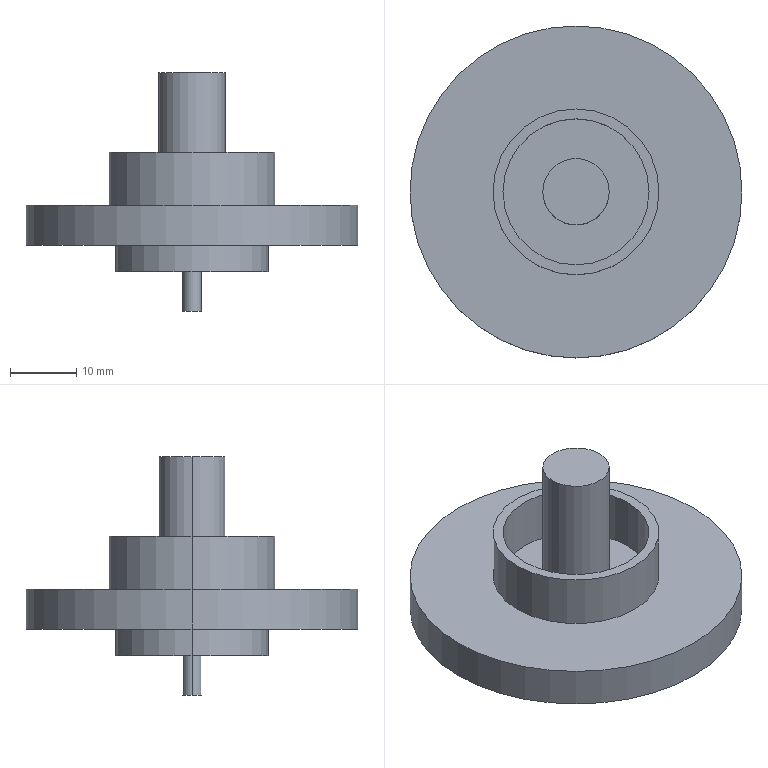Part | SolidWorks | features ICE 4, Extrusion 1 | 1 solid | 22 faces | box 50 x 50 x 36 mm | volume 14585 mm3 | cylinder 14 | plane 8 | commonest cylinder face diameters 2.85 x2 10 x2 20.95 x2 22 x2 23 x2 25 x2
STEP:
#1=CARTESIAN_POINT('',(-1.425,0.,-10.));
#2=VERTEX_POINT('',#1);
#3=CARTESIAN_POINT('',(1.425,0.,-10.));
#4=VERTEX_POINT('',#3);
#5=CARTESIAN_POINT('',(0.,0.,-10.));
#6=DIRECTION('',(0.,0.,-1.));
#7=DIRECTION('',(-1.,0.,0.));
#8=AXIS2_PLACEMENT_3D('',#5,#6,#7);
#9=CIRCLE('',#8,1.425);
#10=EDGE_CURVE('',#2,#4,#9,.T.);
#11=ORIENTED_EDGE('',*,*,#10,.F.);
#12=CARTESIAN_POINT('',(-1.425,0.,0.));
#13=VERTEX_POINT('',#12);
#14=CARTESIAN_POINT('',(-1.425,0.,-10.));
#15=DIRECTION('',(0.,0.,1.));
#16=VECTOR('',#15,1000.);
#17=LINE('',#14,#16);
#18=EDGE_CURVE('',#2,#13,#17,.T.);
#19=ORIENTED_EDGE('',*,*,#18,.T.);
#20=CARTESIAN_POINT('',(1.425,0.,0.));
#21=VERTEX_POINT('',#20);
#22=CARTESIAN_POINT('',(0.,0.,0.));
#23=DIRECTION('',(0.,0.,-1.));
#24=DIRECTION('',(1.,0.,0.));
#25=AXIS2_PLACEMENT_3D('',#22,#23,#24);
#26=CIRCLE('',#25,1.425);
#27=EDGE_CURVE('',#13,#21,#26,.T.);
#28=ORIENTED_EDGE('',*,*,#27,.T.);
#29=CARTESIAN_POINT('',(1.425,0.,-10.));
#30=DIRECTION('',(0.,0.,1.));
#31=VECTOR('',#30,1000.);
#32=LINE('',#29,#31);
#33=EDGE_CURVE('',#4,#21,#32,.T.);
#34=ORIENTED_EDGE('',*,*,#33,.F.);
#35=EDGE_LOOP('',(#11,#19,#28,#34));
#36=FACE_OUTER_BOUND('',#35,.T.);
#37=CARTESIAN_POINT('',(0.,0.,-10.));
#38=DIRECTION('',(0.,0.,1.));
#39=DIRECTION('',(1.,0.,0.));
#40=AXIS2_PLACEMENT_3D('',#37,#38,#39);
#41=CYLINDRICAL_SURFACE('',#40,1.425);
#42=ADVANCED_FACE('',(#36),#41,.T.);
#43=CARTESIAN_POINT('',(10.475,0.,-4.));
#44=VERTEX_POINT('',#43);
#45=CARTESIAN_POINT('',(-10.475,0.,-4.));
#46=VERTEX_POINT('',#45);
#47=CARTESIAN_POINT('',(0.,0.,-4.));
#48=DIRECTION('',(0.,0.,-1.));
#49=DIRECTION('',(-1.,0.,0.));
#50=AXIS2_PLACEMENT_3D('',#47,#48,#49);
#51=CIRCLE('',#50,10.475);
#52=EDGE_CURVE('',#44,#46,#51,.T.);
#53=ORIENTED_EDGE('',*,*,#52,.T.);
#54=CARTESIAN_POINT('',(-10.475,0.,0.));
#55=VERTEX_POINT('',#54);
#56=CARTESIAN_POINT('',(-10.475,0.,-4.));
#57=DIRECTION('',(0.,0.,1.));
#58=VECTOR('',#57,1000.);
#59=LINE('',#56,#58);
#60=EDGE_CURVE('',#46,#55,#59,.T.);
#61=ORIENTED_EDGE('',*,*,#60,.T.);
#62=CARTESIAN_POINT('',(10.475,0.,0.));
#63=VERTEX_POINT('',#62);
#64=CARTESIAN_POINT('',(0.,0.,0.));
#65=DIRECTION('',(0.,0.,-1.));
#66=DIRECTION('',(-1.,0.,0.));
#67=AXIS2_PLACEMENT_3D('',#64,#65,#66);
#68=CIRCLE('',#67,10.475);
#69=EDGE_CURVE('',#63,#55,#68,.T.);
#70=ORIENTED_EDGE('',*,*,#69,.F.);
#71=CARTESIAN_POINT('',(10.475,0.,-4.));
#72=DIRECTION('',(0.,0.,1.));
#73=VECTOR('',#72,1000.);
#74=LINE('',#71,#73);
#75=EDGE_CURVE('',#44,#63,#74,.T.);
#76=ORIENTED_EDGE('',*,*,#75,.F.);
#77=EDGE_LOOP('',(#53,#61,#70,#76));
#78=FACE_OUTER_BOUND('',#77,.T.);
#79=CARTESIAN_POINT('',(0.,0.,-4.));
#80=DIRECTION('',(0.,0.,1.));
#81=DIRECTION('',(1.,0.,0.));
#82=AXIS2_PLACEMENT_3D('',#79,#80,#81);
#83=CYLINDRICAL_SURFACE('',#82,10.475);
#84=ADVANCED_FACE('',(#78),#83,.F.);
#85=CARTESIAN_POINT('',(-11.5,0.,-4.));
#86=VERTEX_POINT('',#85);
#87=CARTESIAN_POINT('',(11.5,0.,-4.));
#88=VERTEX_POINT('',#87);
#89=CARTESIAN_POINT('',(0.,0.,-4.));
#90=DIRECTION('',(0.,0.,-1.));
#91=DIRECTION('',(-1.,0.,0.));
#92=AXIS2_PLACEMENT_3D('',#89,#90,#91);
#93=CIRCLE('',#92,11.5);
#94=EDGE_CURVE('',#86,#88,#93,.T.);
#95=ORIENTED_EDGE('',*,*,#94,.F.);
#96=CARTESIAN_POINT('',(-11.5,0.,0.));
#97=VERTEX_POINT('',#96);
#98=CARTESIAN_POINT('',(-11.5,0.,-4.));
#99=DIRECTION('',(0.,0.,1.));
#100=VECTOR('',#99,1000.);
#101=LINE('',#98,#100);
#102=EDGE_CURVE('',#86,#97,#101,.T.);
#103=ORIENTED_EDGE('',*,*,#102,.T.);
#104=CARTESIAN_POINT('',(11.5,0.,0.));
#105=VERTEX_POINT('',#104);
#106=CARTESIAN_POINT('',(0.,0.,0.));
#107=DIRECTION('',(0.,0.,-1.));
#108=DIRECTION('',(1.,0.,0.));
#109=AXIS2_PLACEMENT_3D('',#106,#107,#108);
#110=CIRCLE('',#109,11.5);
#111=EDGE_CURVE('',#97,#105,#110,.T.);
#112=ORIENTED_EDGE('',*,*,#111,.T.);
#113=CARTESIAN_POINT('',(11.5,0.,-4.));
#114=DIRECTION('',(0.,0.,1.));
#115=VECTOR('',#114,1000.);
#116=LINE('',#113,#115);
#117=EDGE_CURVE('',#88,#105,#116,.T.);
#118=ORIENTED_EDGE('',*,*,#117,.F.);
#119=EDGE_LOOP('',(#95,#103,#112,#118));
#120=FACE_OUTER_BOUND('',#119,.T.);
#121=CARTESIAN_POINT('',(0.,0.,-4.));
#122=DIRECTION('',(0.,0.,1.));
#123=DIRECTION('',(1.,0.,0.));
#124=AXIS2_PLACEMENT_3D('',#121,#122,#123);
#125=CYLINDRICAL_SURFACE('',#124,11.5);
#126=ADVANCED_FACE('',(#120),#125,.T.);
#127=CARTESIAN_POINT('',(5.,0.,26.));
#128=VERTEX_POINT('',#127);
#129=CARTESIAN_POINT('',(-5.,0.,26.));
#130=VERTEX_POINT('',#129);
#131=CARTESIAN_POINT('',(0.,0.,26.));
#132=DIRECTION('',(0.,0.,1.));
#133=DIRECTION('',(1.,0.,0.));
#134=AXIS2_PLACEMENT_3D('',#131,#132,#133);
#135=CIRCLE('',#134,5.);
#136=EDGE_CURVE('',#128,#130,#135,.T.);
#137=ORIENTED_EDGE('',*,*,#136,.F.);
#138=CARTESIAN_POINT('',(5.,0.,6.));
#139=VERTEX_POINT('',#138);
#140=CARTESIAN_POINT('',(5.,0.,26.));
#141=DIRECTION('',(0.,0.,-1.));
#142=VECTOR('',#141,1000.);
#143=LINE('',#140,#142);
#144=EDGE_CURVE('',#128,#139,#143,.T.);
#145=ORIENTED_EDGE('',*,*,#144,.T.);
#146=CARTESIAN_POINT('',(-5.,0.,6.));
#147=VERTEX_POINT('',#146);
#148=CARTESIAN_POINT('',(0.,0.,6.));
#149=DIRECTION('',(0.,0.,1.));
#150=DIRECTION('',(1.,0.,0.));
#151=AXIS2_PLACEMENT_3D('',#148,#149,#150);
#152=CIRCLE('',#151,5.);
#153=EDGE_CURVE('',#139,#147,#152,.T.);
#154=ORIENTED_EDGE('',*,*,#153,.T.);
#155=CARTESIAN_POINT('',(-5.,0.,26.));
#156=DIRECTION('',(0.,0.,-1.));
#157=VECTOR('',#156,1000.);
#158=LINE('',#155,#157);
#159=EDGE_CURVE('',#130,#147,#158,.T.);
#160=ORIENTED_EDGE('',*,*,#159,.F.);
#161=EDGE_LOOP('',(#137,#145,#154,#160));
#162=FACE_OUTER_BOUND('',#161,.T.);
#163=CARTESIAN_POINT('',(0.,0.,26.));
#164=DIRECTION('',(0.,0.,-1.));
#165=DIRECTION('',(-1.,0.,0.));
#166=AXIS2_PLACEMENT_3D('',#163,#164,#165);
#167=CYLINDRICAL_SURFACE('',#166,5.);
#168=ADVANCED_FACE('',(#162),#167,.T.);
#169=CARTESIAN_POINT('',(-11.,0.,14.));
#170=VERTEX_POINT('',#169);
#171=CARTESIAN_POINT('',(11.,0.,14.));
#172=VERTEX_POINT('',#171);
#173=CARTESIAN_POINT('',(0.,0.,14.));
#174=DIRECTION('',(0.,0.,1.));
#175=DIRECTION('',(1.,0.,0.));
#176=AXIS2_PLACEMENT_3D('',#173,#174,#175);
#177=CIRCLE('',#176,11.);
#178=EDGE_CURVE('',#170,#172,#177,.T.);
#179=ORIENTED_EDGE('',*,*,#178,.T.);
#180=CARTESIAN_POINT('',(11.,0.,6.));
#181=VERTEX_POINT('',#180);
#182=CARTESIAN_POINT('',(11.,0.,14.));
#183=DIRECTION('',(0.,0.,-1.));
#184=VECTOR('',#183,1000.);
#185=LINE('',#182,#184);
#186=EDGE_CURVE('',#172,#181,#185,.T.);
#187=ORIENTED_EDGE('',*,*,#186,.T.);
#188=CARTESIAN_POINT('',(-11.,0.,6.));
#189=VERTEX_POINT('',#188);
#190=CARTESIAN_POINT('',(0.,0.,6.));
#191=DIRECTION('',(0.,0.,-1.));
#192=DIRECTION('',(1.,0.,0.));
#193=AXIS2_PLACEMENT_3D('',#190,#191,#192);
#194=CIRCLE('',#193,11.);
#195=EDGE_CURVE('',#181,#189,#194,.T.);
#196=ORIENTED_EDGE('',*,*,#195,.T.);
#197=CARTESIAN_POINT('',(-11.,0.,14.));
#198=DIRECTION('',(0.,0.,-1.));
#199=VECTOR('',#198,1000.);
#200=LINE('',#197,#199);
#201=EDGE_CURVE('',#170,#189,#200,.T.);
#202=ORIENTED_EDGE('',*,*,#201,.F.);
#203=EDGE_LOOP('',(#179,#187,#196,#202));
#204=FACE_OUTER_BOUND('',#203,.T.);
#205=CARTESIAN_POINT('',(0.,0.,14.));
#206=DIRECTION('',(0.,0.,-1.));
#207=DIRECTION('',(-1.,0.,0.));
#208=AXIS2_PLACEMENT_3D('',#205,#206,#207);
#209=CYLINDRICAL_SURFACE('',#208,11.);
#210=ADVANCED_FACE('',(#204),#209,.F.);
#211=CARTESIAN_POINT('',(12.5,0.,14.));
#212=VERTEX_POINT('',#211);
#213=CARTESIAN_POINT('',(-12.5,0.,14.));
#214=VERTEX_POINT('',#213);
#215=CARTESIAN_POINT('',(0.,0.,14.));
#216=DIRECTION('',(0.,0.,1.));
#217=DIRECTION('',(1.,0.,0.));
#218=AXIS2_PLACEMENT_3D('',#215,#216,#217);
#219=CIRCLE('',#218,12.5);
#220=EDGE_CURVE('',#212,#214,#219,.T.);
#221=ORIENTED_EDGE('',*,*,#220,.F.);
#222=CARTESIAN_POINT('',(12.5,0.,6.));
#223=VERTEX_POINT('',#222);
#224=CARTESIAN_POINT('',(12.5,0.,14.));
#225=DIRECTION('',(0.,0.,-1.));
#226=VECTOR('',#225,1000.);
#227=LINE('',#224,#226);
#228=EDGE_CURVE('',#212,#223,#227,.T.);
#229=ORIENTED_EDGE('',*,*,#228,.T.);
#230=CARTESIAN_POINT('',(-12.5,0.,6.));
#231=VERTEX_POINT('',#230);
#232=CARTESIAN_POINT('',(0.,0.,6.));
#233=DIRECTION('',(0.,0.,1.));
#234=DIRECTION('',(1.,0.,0.));
#235=AXIS2_PLACEMENT_3D('',#232,#233,#234);
#236=CIRCLE('',#235,12.5);
#237=EDGE_CURVE('',#223,#231,#236,.T.);
#238=ORIENTED_EDGE('',*,*,#237,.T.);
#239=CARTESIAN_POINT('',(-12.5,0.,14.));
#240=DIRECTION('',(0.,0.,-1.));
#241=VECTOR('',#240,1000.);
#242=LINE('',#239,#241);
#243=EDGE_CURVE('',#214,#231,#242,.T.);
#244=ORIENTED_EDGE('',*,*,#243,.F.);
#245=EDGE_LOOP('',(#221,#229,#238,#244));
#246=FACE_OUTER_BOUND('',#245,.T.);
#247=CARTESIAN_POINT('',(0.,0.,14.));
#248=DIRECTION('',(0.,0.,-1.));
#249=DIRECTION('',(-1.,0.,0.));
#250=AXIS2_PLACEMENT_3D('',#247,#248,#249);
#251=CYLINDRICAL_SURFACE('',#250,12.5);
#252=ADVANCED_FACE('',(#246),#251,.T.);
#253=CARTESIAN_POINT('',(25.,0.,6.));
#254=VERTEX_POINT('',#253);
#255=CARTESIAN_POINT('',(-25.,0.,6.));
#256=VERTEX_POINT('',#255);
#257=CARTESIAN_POINT('',(0.,0.,6.));
#258=DIRECTION('',(0.,0.,1.));
#259=DIRECTION('',(1.,0.,0.));
#260=AXIS2_PLACEMENT_3D('',#257,#258,#259);
#261=CIRCLE('',#260,25.);
#262=EDGE_CURVE('',#254,#256,#261,.T.);
#263=ORIENTED_EDGE('',*,*,#262,.F.);
#264=CARTESIAN_POINT('',(25.,0.,0.));
#265=VERTEX_POINT('',#264);
#266=CARTESIAN_POINT('',(25.,0.,6.));
#267=DIRECTION('',(0.,0.,-1.));
#268=VECTOR('',#267,1000.);
#269=LINE('',#266,#268);
#270=EDGE_CURVE('',#254,#265,#269,.T.);
#271=ORIENTED_EDGE('',*,*,#270,.T.);
#272=CARTESIAN_POINT('',(-25.,0.,0.));
#273=VERTEX_POINT('',#272);
#274=CARTESIAN_POINT('',(0.,0.,0.));
#275=DIRECTION('',(0.,0.,1.));
#276=DIRECTION('',(1.,0.,0.));
#277=AXIS2_PLACEMENT_3D('',#274,#275,#276);
#278=CIRCLE('',#277,25.);
#279=EDGE_CURVE('',#265,#273,#278,.T.);
#280=ORIENTED_EDGE('',*,*,#279,.T.);
#281=CARTESIAN_POINT('',(-25.,0.,6.));
#282=DIRECTION('',(0.,0.,-1.));
#283=VECTOR('',#282,1000.);
#284=LINE('',#281,#283);
#285=EDGE_CURVE('',#256,#273,#284,.T.);
#286=ORIENTED_EDGE('',*,*,#285,.F.);
#287=EDGE_LOOP('',(#263,#271,#280,#286));
#288=FACE_OUTER_BOUND('',#287,.T.);
#289=CARTESIAN_POINT('',(0.,0.,6.));
#290=DIRECTION('',(0.,0.,-1.));
#291=DIRECTION('',(-1.,0.,0.));
#292=AXIS2_PLACEMENT_3D('',#289,#290,#291);
#293=CYLINDRICAL_SURFACE('',#292,25.);
#294=ADVANCED_FACE('',(#288),#293,.T.);
#295=ORIENTED_EDGE('',*,*,#270,.F.);
#296=CARTESIAN_POINT('',(0.,0.,6.));
#297=DIRECTION('',(0.,0.,1.));
#298=DIRECTION('',(1.,0.,0.));
#299=AXIS2_PLACEMENT_3D('',#296,#297,#298);
#300=CIRCLE('',#299,25.);
#301=EDGE_CURVE('',#256,#254,#300,.T.);
#302=ORIENTED_EDGE('',*,*,#301,.F.);
#303=ORIENTED_EDGE('',*,*,#285,.T.);
#304=CARTESIAN_POINT('',(0.,0.,0.));
#305=DIRECTION('',(0.,0.,1.));
#306=DIRECTION('',(1.,0.,0.));
#307=AXIS2_PLACEMENT_3D('',#304,#305,#306);
#308=CIRCLE('',#307,25.);
#309=EDGE_CURVE('',#273,#265,#308,.T.);
#310=ORIENTED_EDGE('',*,*,#309,.T.);
#311=EDGE_LOOP('',(#295,#302,#303,#310));
#312=FACE_OUTER_BOUND('',#311,.T.);
#313=CARTESIAN_POINT('',(0.,0.,6.));
#314=DIRECTION('',(0.,0.,-1.));
#315=DIRECTION('',(-1.,0.,0.));
#316=AXIS2_PLACEMENT_3D('',#313,#314,#315);
#317=CYLINDRICAL_SURFACE('',#316,25.);
#318=ADVANCED_FACE('',(#312),#317,.T.);
#319=CARTESIAN_POINT('',(0.,0.,6.));
#320=DIRECTION('',(0.,0.,1.));
#321=DIRECTION('',(1.,0.,0.));
#322=AXIS2_PLACEMENT_3D('',#319,#320,#321);
#323=CIRCLE('',#322,12.5);
#324=EDGE_CURVE('',#231,#223,#323,.T.);
#325=ORIENTED_EDGE('',*,*,#324,.F.);
#326=ORIENTED_EDGE('',*,*,#237,.F.);
#327=EDGE_LOOP('',(#325,#326));
#328=FACE_BOUND('',#327,.T.);
#329=ORIENTED_EDGE('',*,*,#301,.T.);
#330=ORIENTED_EDGE('',*,*,#262,.T.);
#331=EDGE_LOOP('',(#329,#330));
#332=FACE_OUTER_BOUND('',#331,.T.);
#333=CARTESIAN_POINT('',(0.,0.,6.));
#334=DIRECTION('',(0.,0.,1.));
#335=DIRECTION('',(1.,0.,0.));
#336=AXIS2_PLACEMENT_3D('',#333,#334,#335);
#337=PLANE('',#336);
#338=ADVANCED_FACE('',(#328,#332),#337,.T.);
#339=CARTESIAN_POINT('',(0.,0.,0.));
#340=DIRECTION('',(0.,0.,-1.));
#341=DIRECTION('',(1.,0.,0.));
#342=AXIS2_PLACEMENT_3D('',#339,#340,#341);
#343=CIRCLE('',#342,11.5);
#344=EDGE_CURVE('',#105,#97,#343,.T.);
#345=ORIENTED_EDGE('',*,*,#344,.F.);
#346=ORIENTED_EDGE('',*,*,#111,.F.);
#347=EDGE_LOOP('',(#345,#346));
#348=FACE_BOUND('',#347,.T.);
#349=ORIENTED_EDGE('',*,*,#309,.F.);
#350=ORIENTED_EDGE('',*,*,#279,.F.);
#351=EDGE_LOOP('',(#349,#350));
#352=FACE_OUTER_BOUND('',#351,.T.);
#353=CARTESIAN_POINT('',(0.,0.,0.));
#354=DIRECTION('',(0.,0.,1.));
#355=DIRECTION('',(1.,0.,0.));
#356=AXIS2_PLACEMENT_3D('',#353,#354,#355);
#357=PLANE('',#356);
#358=ADVANCED_FACE('',(#348,#352),#357,.F.);
#359=CARTESIAN_POINT('',(0.,0.,14.));
#360=DIRECTION('',(0.,0.,1.));
#361=DIRECTION('',(1.,0.,0.));
#362=AXIS2_PLACEMENT_3D('',#359,#360,#361);
#363=CIRCLE('',#362,12.5);
#364=EDGE_CURVE('',#214,#212,#363,.T.);
#365=ORIENTED_EDGE('',*,*,#364,.T.);
#366=ORIENTED_EDGE('',*,*,#220,.T.);
#367=EDGE_LOOP('',(#365,#366));
#368=FACE_OUTER_BOUND('',#367,.T.);
#369=ORIENTED_EDGE('',*,*,#178,.F.);
#370=CARTESIAN_POINT('',(0.,0.,14.));
#371=DIRECTION('',(0.,0.,1.));
#372=DIRECTION('',(1.,0.,0.));
#373=AXIS2_PLACEMENT_3D('',#370,#371,#372);
#374=CIRCLE('',#373,11.);
#375=EDGE_CURVE('',#172,#170,#374,.T.);
#376=ORIENTED_EDGE('',*,*,#375,.F.);
#377=EDGE_LOOP('',(#369,#376));
#378=FACE_BOUND('',#377,.T.);
#379=CARTESIAN_POINT('',(0.,0.,14.));
#380=DIRECTION('',(0.,0.,1.));
#381=DIRECTION('',(1.,0.,0.));
#382=AXIS2_PLACEMENT_3D('',#379,#380,#381);
#383=PLANE('',#382);
#384=ADVANCED_FACE('',(#368,#378),#383,.T.);
#385=ORIENTED_EDGE('',*,*,#228,.F.);
#386=ORIENTED_EDGE('',*,*,#364,.F.);
#387=ORIENTED_EDGE('',*,*,#243,.T.);
#388=ORIENTED_EDGE('',*,*,#324,.T.);
#389=EDGE_LOOP('',(#385,#386,#387,#388));
#390=FACE_OUTER_BOUND('',#389,.T.);
#391=CARTESIAN_POINT('',(0.,0.,14.));
#392=DIRECTION('',(0.,0.,-1.));
#393=DIRECTION('',(-1.,0.,0.));
#394=AXIS2_PLACEMENT_3D('',#391,#392,#393);
#395=CYLINDRICAL_SURFACE('',#394,12.5);
#396=ADVANCED_FACE('',(#390),#395,.T.);
#397=ORIENTED_EDGE('',*,*,#186,.F.);
#398=ORIENTED_EDGE('',*,*,#375,.T.);
#399=ORIENTED_EDGE('',*,*,#201,.T.);
#400=CARTESIAN_POINT('',(0.,0.,6.));
#401=DIRECTION('',(0.,0.,-1.));
#402=DIRECTION('',(1.,0.,0.));
#403=AXIS2_PLACEMENT_3D('',#400,#401,#402);
#404=CIRCLE('',#403,11.);
#405=EDGE_CURVE('',#189,#181,#404,.T.);
#406=ORIENTED_EDGE('',*,*,#405,.T.);
#407=EDGE_LOOP('',(#397,#398,#399,#406));
#408=FACE_OUTER_BOUND('',#407,.T.);
#409=CARTESIAN_POINT('',(0.,0.,14.));
#410=DIRECTION('',(0.,0.,-1.));
#411=DIRECTION('',(-1.,0.,0.));
#412=AXIS2_PLACEMENT_3D('',#409,#410,#411);
#413=CYLINDRICAL_SURFACE('',#412,11.);
#414=ADVANCED_FACE('',(#408),#413,.F.);
#415=CARTESIAN_POINT('',(0.,0.,6.));
#416=DIRECTION('',(0.,0.,1.));
#417=DIRECTION('',(1.,0.,0.));
#418=AXIS2_PLACEMENT_3D('',#415,#416,#417);
#419=CIRCLE('',#418,5.);
#420=EDGE_CURVE('',#147,#139,#419,.T.);
#421=ORIENTED_EDGE('',*,*,#420,.F.);
#422=ORIENTED_EDGE('',*,*,#153,.F.);
#423=EDGE_LOOP('',(#421,#422));
#424=FACE_BOUND('',#423,.T.);
#425=ORIENTED_EDGE('',*,*,#405,.F.);
#426=ORIENTED_EDGE('',*,*,#195,.F.);
#427=EDGE_LOOP('',(#425,#426));
#428=FACE_OUTER_BOUND('',#427,.T.);
#429=CARTESIAN_POINT('',(0.,0.,6.));
#430=DIRECTION('',(0.,0.,1.));
#431=DIRECTION('',(1.,0.,0.));
#432=AXIS2_PLACEMENT_3D('',#429,#430,#431);
#433=PLANE('',#432);
#434=ADVANCED_FACE('',(#424,#428),#433,.T.);
#435=ORIENTED_EDGE('',*,*,#144,.F.);
#436=CARTESIAN_POINT('',(0.,0.,26.));
#437=DIRECTION('',(0.,0.,1.));
#438=DIRECTION('',(1.,0.,0.));
#439=AXIS2_PLACEMENT_3D('',#436,#437,#438);
#440=CIRCLE('',#439,5.);
#441=EDGE_CURVE('',#130,#128,#440,.T.);
#442=ORIENTED_EDGE('',*,*,#441,.F.);
#443=ORIENTED_EDGE('',*,*,#159,.T.);
#444=ORIENTED_EDGE('',*,*,#420,.T.);
#445=EDGE_LOOP('',(#435,#442,#443,#444));
#446=FACE_OUTER_BOUND('',#445,.T.);
#447=CARTESIAN_POINT('',(0.,0.,26.));
#448=DIRECTION('',(0.,0.,-1.));
#449=DIRECTION('',(-1.,0.,0.));
#450=AXIS2_PLACEMENT_3D('',#447,#448,#449);
#451=CYLINDRICAL_SURFACE('',#450,5.);
#452=ADVANCED_FACE('',(#446),#451,.T.);
#453=ORIENTED_EDGE('',*,*,#441,.T.);
#454=ORIENTED_EDGE('',*,*,#136,.T.);
#455=EDGE_LOOP('',(#453,#454));
#456=FACE_OUTER_BOUND('',#455,.T.);
#457=CARTESIAN_POINT('',(0.,0.,26.));
#458=DIRECTION('',(0.,0.,1.));
#459=DIRECTION('',(1.,0.,0.));
#460=AXIS2_PLACEMENT_3D('',#457,#458,#459);
#461=PLANE('',#460);
#462=ADVANCED_FACE('',(#456),#461,.T.);
#463=CARTESIAN_POINT('',(0.,0.,-4.));
#464=DIRECTION('',(0.,0.,-1.));
#465=DIRECTION('',(-1.,0.,0.));
#466=AXIS2_PLACEMENT_3D('',#463,#464,#465);
#467=CIRCLE('',#466,11.5);
#468=EDGE_CURVE('',#88,#86,#467,.T.);
#469=ORIENTED_EDGE('',*,*,#468,.T.);
#470=ORIENTED_EDGE('',*,*,#94,.T.);
#471=EDGE_LOOP('',(#469,#470));
#472=FACE_OUTER_BOUND('',#471,.T.);
#473=ORIENTED_EDGE('',*,*,#52,.F.);
#474=CARTESIAN_POINT('',(0.,0.,-4.));
#475=DIRECTION('',(0.,0.,-1.));
#476=DIRECTION('',(-1.,0.,0.));
#477=AXIS2_PLACEMENT_3D('',#474,#475,#476);
#478=CIRCLE('',#477,10.475);
#479=EDGE_CURVE('',#46,#44,#478,.T.);
#480=ORIENTED_EDGE('',*,*,#479,.F.);
#481=EDGE_LOOP('',(#473,#480));
#482=FACE_BOUND('',#481,.T.);
#483=CARTESIAN_POINT('',(0.,0.,-4.));
#484=DIRECTION('',(0.,0.,-1.));
#485=DIRECTION('',(-1.,0.,0.));
#486=AXIS2_PLACEMENT_3D('',#483,#484,#485);
#487=PLANE('',#486);
#488=ADVANCED_FACE('',(#472,#482),#487,.T.);
#489=ORIENTED_EDGE('',*,*,#102,.F.);
#490=ORIENTED_EDGE('',*,*,#468,.F.);
#491=ORIENTED_EDGE('',*,*,#117,.T.);
#492=ORIENTED_EDGE('',*,*,#344,.T.);
#493=EDGE_LOOP('',(#489,#490,#491,#492));
#494=FACE_OUTER_BOUND('',#493,.T.);
#495=CARTESIAN_POINT('',(0.,0.,-4.));
#496=DIRECTION('',(0.,0.,1.));
#497=DIRECTION('',(1.,0.,0.));
#498=AXIS2_PLACEMENT_3D('',#495,#496,#497);
#499=CYLINDRICAL_SURFACE('',#498,11.5);
#500=ADVANCED_FACE('',(#494),#499,.T.);
#501=ORIENTED_EDGE('',*,*,#60,.F.);
#502=ORIENTED_EDGE('',*,*,#479,.T.);
#503=ORIENTED_EDGE('',*,*,#75,.T.);
#504=CARTESIAN_POINT('',(0.,0.,0.));
#505=DIRECTION('',(0.,0.,-1.));
#506=DIRECTION('',(-1.,0.,0.));
#507=AXIS2_PLACEMENT_3D('',#504,#505,#506);
#508=CIRCLE('',#507,10.475);
#509=EDGE_CURVE('',#55,#63,#508,.T.);
#510=ORIENTED_EDGE('',*,*,#509,.F.);
#511=EDGE_LOOP('',(#501,#502,#503,#510));
#512=FACE_OUTER_BOUND('',#511,.T.);
#513=CARTESIAN_POINT('',(0.,0.,-4.));
#514=DIRECTION('',(0.,0.,1.));
#515=DIRECTION('',(1.,0.,0.));
#516=AXIS2_PLACEMENT_3D('',#513,#514,#515);
#517=CYLINDRICAL_SURFACE('',#516,10.475);
#518=ADVANCED_FACE('',(#512),#517,.F.);
#519=CARTESIAN_POINT('',(0.,0.,0.));
#520=DIRECTION('',(0.,0.,-1.));
#521=DIRECTION('',(1.,0.,0.));
#522=AXIS2_PLACEMENT_3D('',#519,#520,#521);
#523=CIRCLE('',#522,1.425);
#524=EDGE_CURVE('',#21,#13,#523,.T.);
#525=ORIENTED_EDGE('',*,*,#524,.F.);
#526=ORIENTED_EDGE('',*,*,#27,.F.);
#527=EDGE_LOOP('',(#525,#526));
#528=FACE_BOUND('',#527,.T.);
#529=ORIENTED_EDGE('',*,*,#69,.T.);
#530=ORIENTED_EDGE('',*,*,#509,.T.);
#531=EDGE_LOOP('',(#529,#530));
#532=FACE_OUTER_BOUND('',#531,.T.);
#533=CARTESIAN_POINT('',(0.,0.,0.));
#534=DIRECTION('',(0.,0.,1.));
#535=DIRECTION('',(1.,0.,0.));
#536=AXIS2_PLACEMENT_3D('',#533,#534,#535);
#537=PLANE('',#536);
#538=ADVANCED_FACE('',(#528,#532),#537,.F.);
#539=ORIENTED_EDGE('',*,*,#18,.F.);
#540=CARTESIAN_POINT('',(0.,0.,-10.));
#541=DIRECTION('',(0.,0.,-1.));
#542=DIRECTION('',(-1.,0.,0.));
#543=AXIS2_PLACEMENT_3D('',#540,#541,#542);
#544=CIRCLE('',#543,1.425);
#545=EDGE_CURVE('',#4,#2,#544,.T.);
#546=ORIENTED_EDGE('',*,*,#545,.F.);
#547=ORIENTED_EDGE('',*,*,#33,.T.);
#548=ORIENTED_EDGE('',*,*,#524,.T.);
#549=EDGE_LOOP('',(#539,#546,#547,#548));
#550=FACE_OUTER_BOUND('',#549,.T.);
#551=CARTESIAN_POINT('',(0.,0.,-10.));
#552=DIRECTION('',(0.,0.,1.));
#553=DIRECTION('',(1.,0.,0.));
#554=AXIS2_PLACEMENT_3D('',#551,#552,#553);
#555=CYLINDRICAL_SURFACE('',#554,1.425);
#556=ADVANCED_FACE('',(#550),#555,.T.);
#557=ORIENTED_EDGE('',*,*,#545,.T.);
#558=ORIENTED_EDGE('',*,*,#10,.T.);
#559=EDGE_LOOP('',(#557,#558));
#560=FACE_OUTER_BOUND('',#559,.T.);
#561=CARTESIAN_POINT('',(0.,0.,-10.));
#562=DIRECTION('',(0.,0.,-1.));
#563=DIRECTION('',(-1.,0.,0.));
#564=AXIS2_PLACEMENT_3D('',#561,#562,#563);
#565=PLANE('',#564);
#566=ADVANCED_FACE('',(#560),#565,.T.);
#567=CLOSED_SHELL('',(#42,#84,#126,#168,#210,#252,#294,#318,#338,#358,#384,#396,#414,#434,#452,#462,#488,#500,#518,#538,#556,#566));
#568=MANIFOLD_SOLID_BREP('',#567);
#569=CARTESIAN_POINT('',(0.,0.,0.));
#570=DIRECTION('',(0.,0.,1.));
#571=DIRECTION('',(1.,0.,0.));
#572=AXIS2_PLACEMENT_3D('',#569,#570,#571);
#573=(LENGTH_UNIT()NAMED_UNIT(*)SI_UNIT(.MILLI.,.METRE.));
#574=UNCERTAINTY_MEASURE_WITH_UNIT(LENGTH_MEASURE(0.00001),#573,'','');
#575=(NAMED_UNIT(*)PLANE_ANGLE_UNIT()SI_UNIT($,.RADIAN.));
#576=(NAMED_UNIT(*)SI_UNIT($,.STERADIAN.)SOLID_ANGLE_UNIT());
#577=(GEOMETRIC_REPRESENTATION_CONTEXT(3)GLOBAL_UNCERTAINTY_ASSIGNED_CONTEXT((#574))GLOBAL_UNIT_ASSIGNED_CONTEXT((#573,#575,#576))REPRESENTATION_CONTEXT('',''));
#578=ADVANCED_BREP_SHAPE_REPRESENTATION('',(#568,#572),#577);